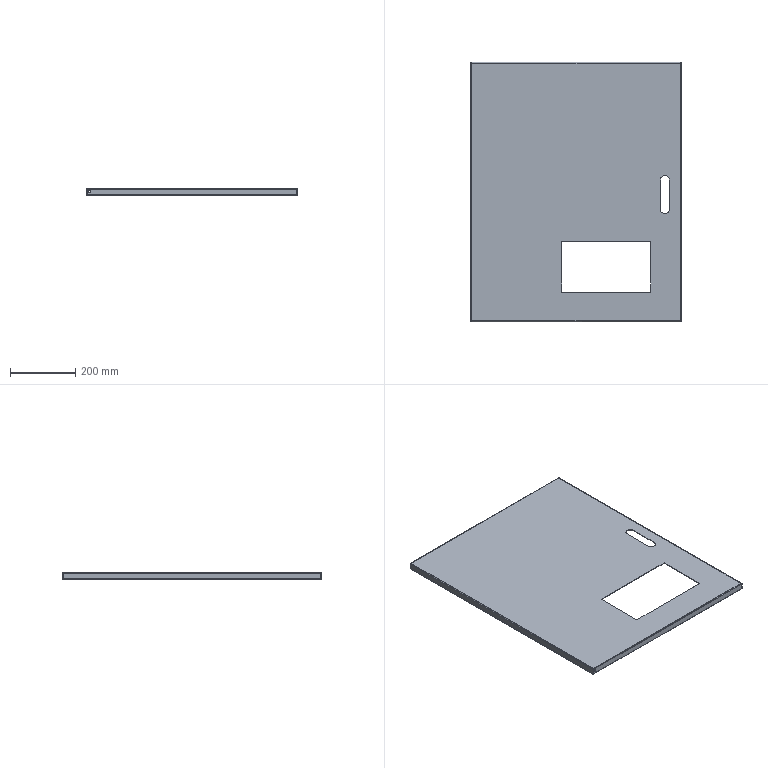Part | STEP file | Left Door | 1 solid | 106 faces | box 645 x 795 x 21 mm | volume 1111473 mm3 | plane 68 | cylinder 22 | spline 16 | commonest cylinder face diameters 0.2 x8 4.2 x8 7 x4 27 x2